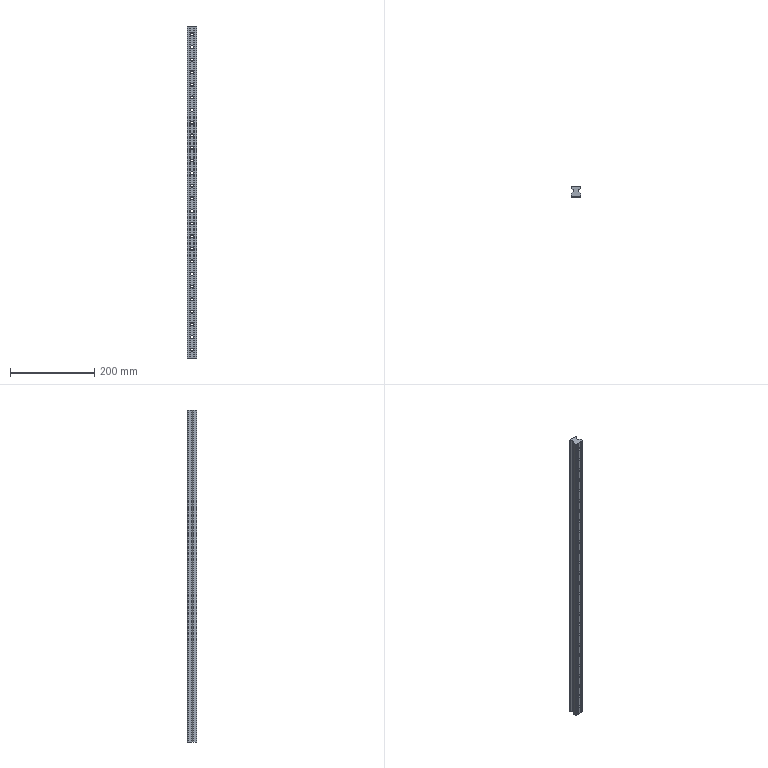Part | STEP file | 2026.6.15-Main Assembly图.sldasm-Part-11 | 1 solid | 168 faces | box 23 x 23.6 x 790 mm | volume 320754 mm3 | cylinder 112 | plane 56 | commonest cylinder face diameters 7 x52 11 x52 1.629 x8